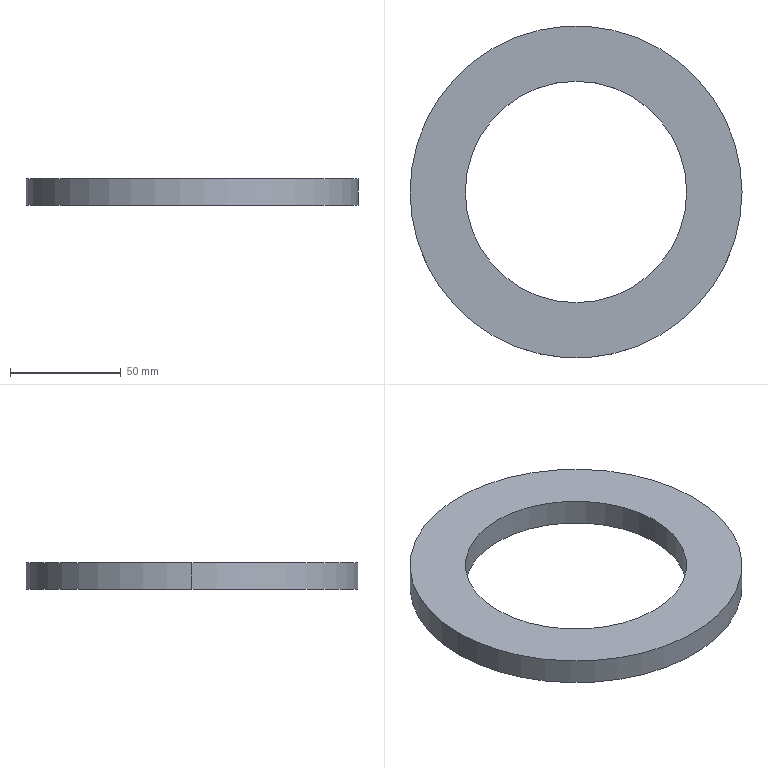Part | SolidWorks | features Extrusion 1 | 1 solid | 6 faces | box 150 x 150 x 12 mm | volume 117810 mm3 | cylinder 4 | plane 2 | commonest cylinder face diameters 100 x2 150 x2
STEP:
#1=CARTESIAN_POINT('',(-50.,0.,12.));
#2=VERTEX_POINT('',#1);
#3=CARTESIAN_POINT('',(50.,0.,12.));
#4=VERTEX_POINT('',#3);
#5=CARTESIAN_POINT('',(0.,0.,12.));
#6=DIRECTION('',(0.,0.,1.));
#7=DIRECTION('',(1.,0.,0.));
#8=AXIS2_PLACEMENT_3D('',#5,#6,#7);
#9=CIRCLE('',#8,50.);
#10=EDGE_CURVE('',#2,#4,#9,.T.);
#11=ORIENTED_EDGE('',*,*,#10,.T.);
#12=CARTESIAN_POINT('',(50.,0.,0.));
#13=VERTEX_POINT('',#12);
#14=CARTESIAN_POINT('',(50.,0.,12.));
#15=DIRECTION('',(0.,0.,-1.));
#16=VECTOR('',#15,1000.);
#17=LINE('',#14,#16);
#18=EDGE_CURVE('',#4,#13,#17,.T.);
#19=ORIENTED_EDGE('',*,*,#18,.T.);
#20=CARTESIAN_POINT('',(-50.,0.,0.));
#21=VERTEX_POINT('',#20);
#22=CARTESIAN_POINT('',(0.,0.,0.));
#23=DIRECTION('',(0.,0.,1.));
#24=DIRECTION('',(1.,0.,0.));
#25=AXIS2_PLACEMENT_3D('',#22,#23,#24);
#26=CIRCLE('',#25,50.);
#27=EDGE_CURVE('',#21,#13,#26,.T.);
#28=ORIENTED_EDGE('',*,*,#27,.F.);
#29=CARTESIAN_POINT('',(-50.,0.,12.));
#30=DIRECTION('',(0.,0.,-1.));
#31=VECTOR('',#30,1000.);
#32=LINE('',#29,#31);
#33=EDGE_CURVE('',#2,#21,#32,.T.);
#34=ORIENTED_EDGE('',*,*,#33,.F.);
#35=EDGE_LOOP('',(#11,#19,#28,#34));
#36=FACE_OUTER_BOUND('',#35,.T.);
#37=CARTESIAN_POINT('',(0.,0.,12.));
#38=DIRECTION('',(0.,0.,-1.));
#39=DIRECTION('',(-1.,0.,0.));
#40=AXIS2_PLACEMENT_3D('',#37,#38,#39);
#41=CYLINDRICAL_SURFACE('',#40,50.);
#42=ADVANCED_FACE('',(#36),#41,.F.);
#43=CARTESIAN_POINT('',(75.,0.,12.));
#44=VERTEX_POINT('',#43);
#45=CARTESIAN_POINT('',(-75.,0.,12.));
#46=VERTEX_POINT('',#45);
#47=CARTESIAN_POINT('',(0.,0.,12.));
#48=DIRECTION('',(0.,0.,1.));
#49=DIRECTION('',(1.,0.,0.));
#50=AXIS2_PLACEMENT_3D('',#47,#48,#49);
#51=CIRCLE('',#50,75.);
#52=EDGE_CURVE('',#44,#46,#51,.T.);
#53=ORIENTED_EDGE('',*,*,#52,.F.);
#54=CARTESIAN_POINT('',(75.,0.,0.));
#55=VERTEX_POINT('',#54);
#56=CARTESIAN_POINT('',(75.,0.,12.));
#57=DIRECTION('',(0.,0.,-1.));
#58=VECTOR('',#57,1000.);
#59=LINE('',#56,#58);
#60=EDGE_CURVE('',#44,#55,#59,.T.);
#61=ORIENTED_EDGE('',*,*,#60,.T.);
#62=CARTESIAN_POINT('',(-75.,0.,0.));
#63=VERTEX_POINT('',#62);
#64=CARTESIAN_POINT('',(0.,0.,0.));
#65=DIRECTION('',(0.,0.,1.));
#66=DIRECTION('',(1.,0.,0.));
#67=AXIS2_PLACEMENT_3D('',#64,#65,#66);
#68=CIRCLE('',#67,75.);
#69=EDGE_CURVE('',#55,#63,#68,.T.);
#70=ORIENTED_EDGE('',*,*,#69,.T.);
#71=CARTESIAN_POINT('',(-75.,0.,12.));
#72=DIRECTION('',(0.,0.,-1.));
#73=VECTOR('',#72,1000.);
#74=LINE('',#71,#73);
#75=EDGE_CURVE('',#46,#63,#74,.T.);
#76=ORIENTED_EDGE('',*,*,#75,.F.);
#77=EDGE_LOOP('',(#53,#61,#70,#76));
#78=FACE_OUTER_BOUND('',#77,.T.);
#79=CARTESIAN_POINT('',(0.,0.,12.));
#80=DIRECTION('',(0.,0.,-1.));
#81=DIRECTION('',(-1.,0.,0.));
#82=AXIS2_PLACEMENT_3D('',#79,#80,#81);
#83=CYLINDRICAL_SURFACE('',#82,75.);
#84=ADVANCED_FACE('',(#78),#83,.T.);
#85=CARTESIAN_POINT('',(0.,0.,12.));
#86=DIRECTION('',(0.,0.,1.));
#87=DIRECTION('',(1.,0.,0.));
#88=AXIS2_PLACEMENT_3D('',#85,#86,#87);
#89=CIRCLE('',#88,75.);
#90=EDGE_CURVE('',#46,#44,#89,.T.);
#91=ORIENTED_EDGE('',*,*,#90,.T.);
#92=ORIENTED_EDGE('',*,*,#52,.T.);
#93=EDGE_LOOP('',(#91,#92));
#94=FACE_OUTER_BOUND('',#93,.T.);
#95=ORIENTED_EDGE('',*,*,#10,.F.);
#96=CARTESIAN_POINT('',(0.,0.,12.));
#97=DIRECTION('',(0.,0.,1.));
#98=DIRECTION('',(1.,0.,0.));
#99=AXIS2_PLACEMENT_3D('',#96,#97,#98);
#100=CIRCLE('',#99,50.);
#101=EDGE_CURVE('',#4,#2,#100,.T.);
#102=ORIENTED_EDGE('',*,*,#101,.F.);
#103=EDGE_LOOP('',(#95,#102));
#104=FACE_BOUND('',#103,.T.);
#105=CARTESIAN_POINT('',(0.,0.,12.));
#106=DIRECTION('',(0.,0.,1.));
#107=DIRECTION('',(1.,0.,0.));
#108=AXIS2_PLACEMENT_3D('',#105,#106,#107);
#109=PLANE('',#108);
#110=ADVANCED_FACE('',(#94,#104),#109,.T.);
#111=CARTESIAN_POINT('',(0.,0.,0.));
#112=DIRECTION('',(0.,0.,1.));
#113=DIRECTION('',(1.,0.,0.));
#114=AXIS2_PLACEMENT_3D('',#111,#112,#113);
#115=CIRCLE('',#114,75.);
#116=EDGE_CURVE('',#63,#55,#115,.T.);
#117=ORIENTED_EDGE('',*,*,#116,.F.);
#118=ORIENTED_EDGE('',*,*,#69,.F.);
#119=EDGE_LOOP('',(#117,#118));
#120=FACE_OUTER_BOUND('',#119,.T.);
#121=ORIENTED_EDGE('',*,*,#27,.T.);
#122=CARTESIAN_POINT('',(0.,0.,0.));
#123=DIRECTION('',(0.,0.,1.));
#124=DIRECTION('',(1.,0.,0.));
#125=AXIS2_PLACEMENT_3D('',#122,#123,#124);
#126=CIRCLE('',#125,50.);
#127=EDGE_CURVE('',#13,#21,#126,.T.);
#128=ORIENTED_EDGE('',*,*,#127,.T.);
#129=EDGE_LOOP('',(#121,#128));
#130=FACE_BOUND('',#129,.T.);
#131=CARTESIAN_POINT('',(0.,0.,0.));
#132=DIRECTION('',(0.,0.,1.));
#133=DIRECTION('',(1.,0.,0.));
#134=AXIS2_PLACEMENT_3D('',#131,#132,#133);
#135=PLANE('',#134);
#136=ADVANCED_FACE('',(#120,#130),#135,.F.);
#137=ORIENTED_EDGE('',*,*,#60,.F.);
#138=ORIENTED_EDGE('',*,*,#90,.F.);
#139=ORIENTED_EDGE('',*,*,#75,.T.);
#140=ORIENTED_EDGE('',*,*,#116,.T.);
#141=EDGE_LOOP('',(#137,#138,#139,#140));
#142=FACE_OUTER_BOUND('',#141,.T.);
#143=CARTESIAN_POINT('',(0.,0.,12.));
#144=DIRECTION('',(0.,0.,-1.));
#145=DIRECTION('',(-1.,0.,0.));
#146=AXIS2_PLACEMENT_3D('',#143,#144,#145);
#147=CYLINDRICAL_SURFACE('',#146,75.);
#148=ADVANCED_FACE('',(#142),#147,.T.);
#149=ORIENTED_EDGE('',*,*,#18,.F.);
#150=ORIENTED_EDGE('',*,*,#101,.T.);
#151=ORIENTED_EDGE('',*,*,#33,.T.);
#152=ORIENTED_EDGE('',*,*,#127,.F.);
#153=EDGE_LOOP('',(#149,#150,#151,#152));
#154=FACE_OUTER_BOUND('',#153,.T.);
#155=CARTESIAN_POINT('',(0.,0.,12.));
#156=DIRECTION('',(0.,0.,-1.));
#157=DIRECTION('',(-1.,0.,0.));
#158=AXIS2_PLACEMENT_3D('',#155,#156,#157);
#159=CYLINDRICAL_SURFACE('',#158,50.);
#160=ADVANCED_FACE('',(#154),#159,.F.);
#161=CLOSED_SHELL('',(#42,#84,#110,#136,#148,#160));
#162=MANIFOLD_SOLID_BREP('',#161);
#163=CARTESIAN_POINT('',(0.,0.,0.));
#164=DIRECTION('',(0.,0.,1.));
#165=DIRECTION('',(1.,0.,0.));
#166=AXIS2_PLACEMENT_3D('',#163,#164,#165);
#167=(LENGTH_UNIT()NAMED_UNIT(*)SI_UNIT(.MILLI.,.METRE.));
#168=UNCERTAINTY_MEASURE_WITH_UNIT(LENGTH_MEASURE(0.00001),#167,'','');
#169=(NAMED_UNIT(*)PLANE_ANGLE_UNIT()SI_UNIT($,.RADIAN.));
#170=(NAMED_UNIT(*)SI_UNIT($,.STERADIAN.)SOLID_ANGLE_UNIT());
#171=(GEOMETRIC_REPRESENTATION_CONTEXT(3)GLOBAL_UNCERTAINTY_ASSIGNED_CONTEXT((#168))GLOBAL_UNIT_ASSIGNED_CONTEXT((#167,#169,#170))REPRESENTATION_CONTEXT('',''));
#172=ADVANCED_BREP_SHAPE_REPRESENTATION('',(#162,#166),#171);